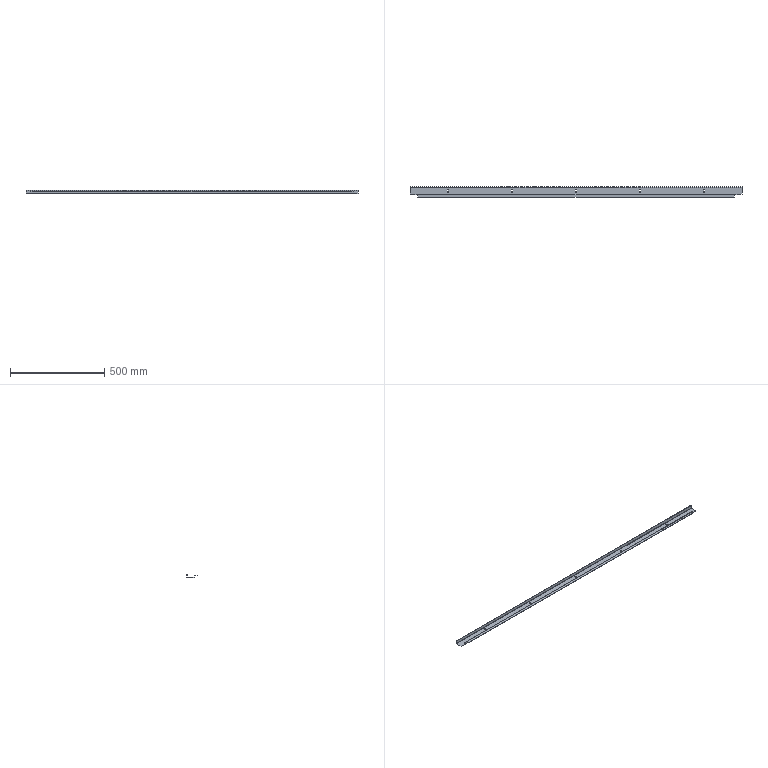Part | SolidWorks | features ICE 5, EdgeFlange 3, FlatPattern 1, SMBaseFlange 1, SheetMetal 1 | 1 solid | 50 faces | box 1760 x 53.5 x 18 mm | volume 208432 mm3 | plane 34 | cylinder 16 | commonest cylinder face diameters 7 x10 2 x3 5 x3
STEP:
#1=CARTESIAN_POINT('',(-855.,-20.,1.));
#2=VERTEX_POINT('',#1);
#3=CARTESIAN_POINT('',(-855.,-20.,10.));
#4=VERTEX_POINT('',#3);
#5=CARTESIAN_POINT('',(-855.,-20.,-1.5));
#6=DIRECTION('',(0.,0.,1.));
#7=VECTOR('',#6,1000.);
#8=LINE('',#5,#7);
#9=EDGE_CURVE('',#2,#4,#8,.T.);
#10=ORIENTED_EDGE('',*,*,#9,.F.);
#11=CARTESIAN_POINT('',(855.,-20.,1.));
#12=VERTEX_POINT('',#11);
#13=CARTESIAN_POINT('',(-880.,-20.,1.));
#14=DIRECTION('',(-1.,0.,0.));
#15=VECTOR('',#14,1000.);
#16=LINE('',#13,#15);
#17=EDGE_CURVE('',#12,#2,#16,.T.);
#18=ORIENTED_EDGE('',*,*,#17,.F.);
#19=CARTESIAN_POINT('',(855.,-20.,10.));
#20=VERTEX_POINT('',#19);
#21=CARTESIAN_POINT('',(855.,-20.,-1.5));
#22=DIRECTION('',(0.,0.,-1.));
#23=VECTOR('',#22,1000.);
#24=LINE('',#21,#23);
#25=EDGE_CURVE('',#20,#12,#24,.T.);
#26=ORIENTED_EDGE('',*,*,#25,.F.);
#27=CARTESIAN_POINT('',(840.,-20.,10.));
#28=VERTEX_POINT('',#27);
#29=CARTESIAN_POINT('',(880.,-20.,10.));
#30=DIRECTION('',(-1.,0.,0.));
#31=VECTOR('',#30,1000.);
#32=LINE('',#29,#31);
#33=EDGE_CURVE('',#20,#28,#32,.T.);
#34=ORIENTED_EDGE('',*,*,#33,.T.);
#35=CARTESIAN_POINT('',(-840.,-20.,10.));
#36=VERTEX_POINT('',#35);
#37=CARTESIAN_POINT('',(-880.,-20.,10.));
#38=DIRECTION('',(1.,0.,0.));
#39=VECTOR('',#38,1000.);
#40=LINE('',#37,#39);
#41=EDGE_CURVE('',#36,#28,#40,.T.);
#42=ORIENTED_EDGE('',*,*,#41,.F.);
#43=CARTESIAN_POINT('',(-880.,-20.,10.));
#44=DIRECTION('',(1.,0.,0.));
#45=VECTOR('',#44,1000.);
#46=LINE('',#43,#45);
#47=EDGE_CURVE('',#4,#36,#46,.T.);
#48=ORIENTED_EDGE('',*,*,#47,.F.);
#49=EDGE_LOOP('',(#10,#18,#26,#34,#42,#48));
#50=FACE_OUTER_BOUND('',#49,.T.);
#51=CARTESIAN_POINT('',(880.,-20.,0.));
#52=DIRECTION('',(0.,1.,0.));
#53=DIRECTION('',(0.,0.,1.));
#54=AXIS2_PLACEMENT_3D('',#51,#52,#53);
#55=PLANE('',#54);
#56=ADVANCED_FACE('',(#50),#55,.F.);
#57=CARTESIAN_POINT('',(-855.,-18.5,1.));
#58=VERTEX_POINT('',#57);
#59=CARTESIAN_POINT('',(855.,-18.5,1.));
#60=VERTEX_POINT('',#59);
#61=CARTESIAN_POINT('',(-880.,-18.5,1.));
#62=DIRECTION('',(1.,0.,0.));
#63=VECTOR('',#62,1000.);
#64=LINE('',#61,#63);
#65=EDGE_CURVE('',#58,#60,#64,.T.);
#66=ORIENTED_EDGE('',*,*,#65,.F.);
#67=CARTESIAN_POINT('',(-855.,-18.5,10.));
#68=VERTEX_POINT('',#67);
#69=CARTESIAN_POINT('',(-855.,-18.5,0.));
#70=DIRECTION('',(0.,0.,1.));
#71=VECTOR('',#70,1000.);
#72=LINE('',#69,#71);
#73=EDGE_CURVE('',#58,#68,#72,.T.);
#74=ORIENTED_EDGE('',*,*,#73,.T.);
#75=CARTESIAN_POINT('',(-840.,-18.5,10.));
#76=VERTEX_POINT('',#75);
#77=CARTESIAN_POINT('',(-880.,-18.5,10.));
#78=DIRECTION('',(1.,0.,0.));
#79=VECTOR('',#78,1000.);
#80=LINE('',#77,#79);
#81=EDGE_CURVE('',#68,#76,#80,.T.);
#82=ORIENTED_EDGE('',*,*,#81,.T.);
#83=CARTESIAN_POINT('',(840.,-18.5,10.));
#84=VERTEX_POINT('',#83);
#85=CARTESIAN_POINT('',(-880.,-18.5,10.));
#86=DIRECTION('',(1.,0.,0.));
#87=VECTOR('',#86,1000.);
#88=LINE('',#85,#87);
#89=EDGE_CURVE('',#76,#84,#88,.T.);
#90=ORIENTED_EDGE('',*,*,#89,.T.);
#91=CARTESIAN_POINT('',(855.,-18.5,10.));
#92=VERTEX_POINT('',#91);
#93=CARTESIAN_POINT('',(840.,-18.5,10.));
#94=DIRECTION('',(1.,0.,0.));
#95=VECTOR('',#94,1000.);
#96=LINE('',#93,#95);
#97=EDGE_CURVE('',#84,#92,#96,.T.);
#98=ORIENTED_EDGE('',*,*,#97,.T.);
#99=CARTESIAN_POINT('',(855.,-18.5,0.));
#100=DIRECTION('',(0.,0.,1.));
#101=VECTOR('',#100,1000.);
#102=LINE('',#99,#101);
#103=EDGE_CURVE('',#60,#92,#102,.T.);
#104=ORIENTED_EDGE('',*,*,#103,.F.);
#105=EDGE_LOOP('',(#66,#74,#82,#90,#98,#104));
#106=FACE_OUTER_BOUND('',#105,.T.);
#107=CARTESIAN_POINT('',(880.,-18.5,0.));
#108=DIRECTION('',(0.,1.,0.));
#109=DIRECTION('',(0.,0.,1.));
#110=AXIS2_PLACEMENT_3D('',#107,#108,#109);
#111=PLANE('',#110);
#112=ADVANCED_FACE('',(#106),#111,.T.);
#113=ORIENTED_EDGE('',*,*,#17,.T.);
#114=CARTESIAN_POINT('',(-855.,-17.5,-1.5));
#115=VERTEX_POINT('',#114);
#116=CARTESIAN_POINT('',(-855.,-17.5,1.));
#117=DIRECTION('',(1.,0.,0.));
#118=DIRECTION('',(0.,0.,1.));
#119=AXIS2_PLACEMENT_3D('',#116,#117,#118);
#120=CIRCLE('',#119,2.5);
#121=EDGE_CURVE('',#2,#115,#120,.T.);
#122=ORIENTED_EDGE('',*,*,#121,.T.);
#123=CARTESIAN_POINT('',(855.,-17.5,-1.5));
#124=VERTEX_POINT('',#123);
#125=CARTESIAN_POINT('',(880.,-17.5,-1.5));
#126=DIRECTION('',(-1.,0.,0.));
#127=VECTOR('',#126,1000.);
#128=LINE('',#125,#127);
#129=EDGE_CURVE('',#124,#115,#128,.T.);
#130=ORIENTED_EDGE('',*,*,#129,.F.);
#131=CARTESIAN_POINT('',(855.,-17.5,1.));
#132=DIRECTION('',(1.,0.,0.));
#133=DIRECTION('',(0.,0.,1.));
#134=AXIS2_PLACEMENT_3D('',#131,#132,#133);
#135=CIRCLE('',#134,2.5);
#136=EDGE_CURVE('',#12,#124,#135,.T.);
#137=ORIENTED_EDGE('',*,*,#136,.F.);
#138=EDGE_LOOP('',(#113,#122,#130,#137));
#139=FACE_OUTER_BOUND('',#138,.T.);
#140=CARTESIAN_POINT('',(880.,-17.5,1.));
#141=DIRECTION('',(1.,0.,0.));
#142=DIRECTION('',(0.,-1.,0.));
#143=AXIS2_PLACEMENT_3D('',#140,#141,#142);
#144=CYLINDRICAL_SURFACE('',#143,2.5);
#145=ADVANCED_FACE('',(#139),#144,.T.);
#146=CARTESIAN_POINT('',(-855.,-17.5,0.));
#147=VERTEX_POINT('',#146);
#148=CARTESIAN_POINT('',(-855.,-17.5,1.));
#149=DIRECTION('',(1.,0.,0.));
#150=DIRECTION('',(0.,0.,1.));
#151=AXIS2_PLACEMENT_3D('',#148,#149,#150);
#152=CIRCLE('',#151,1.);
#153=EDGE_CURVE('',#58,#147,#152,.T.);
#154=ORIENTED_EDGE('',*,*,#153,.F.);
#155=ORIENTED_EDGE('',*,*,#65,.T.);
#156=CARTESIAN_POINT('',(855.,-17.5,0.));
#157=VERTEX_POINT('',#156);
#158=CARTESIAN_POINT('',(855.,-17.5,1.));
#159=DIRECTION('',(1.,0.,0.));
#160=DIRECTION('',(0.,0.,1.));
#161=AXIS2_PLACEMENT_3D('',#158,#159,#160);
#162=CIRCLE('',#161,1.);
#163=EDGE_CURVE('',#60,#157,#162,.T.);
#164=ORIENTED_EDGE('',*,*,#163,.T.);
#165=CARTESIAN_POINT('',(880.,-17.5,0.));
#166=DIRECTION('',(-1.,0.,0.));
#167=VECTOR('',#166,1000.);
#168=LINE('',#165,#167);
#169=EDGE_CURVE('',#157,#147,#168,.T.);
#170=ORIENTED_EDGE('',*,*,#169,.T.);
#171=EDGE_LOOP('',(#154,#155,#164,#170));
#172=FACE_OUTER_BOUND('',#171,.T.);
#173=CARTESIAN_POINT('',(880.,-17.5,1.));
#174=DIRECTION('',(1.,0.,0.));
#175=DIRECTION('',(0.,-1.,0.));
#176=AXIS2_PLACEMENT_3D('',#173,#174,#175);
#177=CYLINDRICAL_SURFACE('',#176,1.);
#178=ADVANCED_FACE('',(#172),#177,.F.);
#179=CARTESIAN_POINT('',(-855.,-17.5,10.));
#180=DIRECTION('',(0.,1.,0.));
#181=VECTOR('',#180,1000.);
#182=LINE('',#179,#181);
#183=EDGE_CURVE('',#4,#68,#182,.T.);
#184=ORIENTED_EDGE('',*,*,#183,.F.);
#185=ORIENTED_EDGE('',*,*,#47,.T.);
#186=CARTESIAN_POINT('',(-840.,-18.5,10.));
#187=DIRECTION('',(0.,-1.,0.));
#188=VECTOR('',#187,1000.);
#189=LINE('',#186,#188);
#190=EDGE_CURVE('',#76,#36,#189,.T.);
#191=ORIENTED_EDGE('',*,*,#190,.F.);
#192=ORIENTED_EDGE('',*,*,#81,.F.);
#193=EDGE_LOOP('',(#184,#185,#191,#192));
#194=FACE_OUTER_BOUND('',#193,.T.);
#195=CARTESIAN_POINT('',(-840.,-18.5,10.));
#196=DIRECTION('',(0.,0.,-1.));
#197=DIRECTION('',(0.,1.,0.));
#198=AXIS2_PLACEMENT_3D('',#195,#196,#197);
#199=PLANE('',#198);
#200=ADVANCED_FACE('',(#194),#199,.F.);
#201=CARTESIAN_POINT('',(840.,-21.,12.5));
#202=VERTEX_POINT('',#201);
#203=CARTESIAN_POINT('',(840.,-21.,10.));
#204=DIRECTION('',(1.,0.,0.));
#205=DIRECTION('',(0.,0.,1.));
#206=AXIS2_PLACEMENT_3D('',#203,#204,#205);
#207=CIRCLE('',#206,2.5);
#208=EDGE_CURVE('',#84,#202,#207,.T.);
#209=ORIENTED_EDGE('',*,*,#208,.F.);
#210=ORIENTED_EDGE('',*,*,#89,.F.);
#211=CARTESIAN_POINT('',(-840.,-21.,12.5));
#212=VERTEX_POINT('',#211);
#213=CARTESIAN_POINT('',(-840.,-21.,10.));
#214=DIRECTION('',(1.,0.,0.));
#215=DIRECTION('',(0.,0.,1.));
#216=AXIS2_PLACEMENT_3D('',#213,#214,#215);
#217=CIRCLE('',#216,2.5);
#218=EDGE_CURVE('',#76,#212,#217,.T.);
#219=ORIENTED_EDGE('',*,*,#218,.T.);
#220=CARTESIAN_POINT('',(880.,-21.,12.5));
#221=DIRECTION('',(1.,0.,0.));
#222=VECTOR('',#221,1000.);
#223=LINE('',#220,#222);
#224=EDGE_CURVE('',#212,#202,#223,.T.);
#225=ORIENTED_EDGE('',*,*,#224,.T.);
#226=EDGE_LOOP('',(#209,#210,#219,#225));
#227=FACE_OUTER_BOUND('',#226,.T.);
#228=CARTESIAN_POINT('',(-880.,-21.,10.));
#229=DIRECTION('',(-1.,0.,0.));
#230=DIRECTION('',(0.,0.,1.));
#231=AXIS2_PLACEMENT_3D('',#228,#229,#230);
#232=CYLINDRICAL_SURFACE('',#231,2.5);
#233=ADVANCED_FACE('',(#227),#232,.T.);
#234=ORIENTED_EDGE('',*,*,#41,.T.);
#235=CARTESIAN_POINT('',(840.,-21.,11.));
#236=VERTEX_POINT('',#235);
#237=CARTESIAN_POINT('',(840.,-21.,10.));
#238=DIRECTION('',(1.,0.,0.));
#239=DIRECTION('',(0.,0.,1.));
#240=AXIS2_PLACEMENT_3D('',#237,#238,#239);
#241=CIRCLE('',#240,1.);
#242=EDGE_CURVE('',#28,#236,#241,.T.);
#243=ORIENTED_EDGE('',*,*,#242,.T.);
#244=CARTESIAN_POINT('',(-840.,-21.,11.));
#245=VERTEX_POINT('',#244);
#246=CARTESIAN_POINT('',(880.,-21.,11.));
#247=DIRECTION('',(-1.,0.,0.));
#248=VECTOR('',#247,1000.);
#249=LINE('',#246,#248);
#250=EDGE_CURVE('',#236,#245,#249,.T.);
#251=ORIENTED_EDGE('',*,*,#250,.T.);
#252=CARTESIAN_POINT('',(-840.,-21.,10.));
#253=DIRECTION('',(1.,0.,0.));
#254=DIRECTION('',(0.,0.,1.));
#255=AXIS2_PLACEMENT_3D('',#252,#253,#254);
#256=CIRCLE('',#255,1.);
#257=EDGE_CURVE('',#36,#245,#256,.T.);
#258=ORIENTED_EDGE('',*,*,#257,.F.);
#259=EDGE_LOOP('',(#234,#243,#251,#258));
#260=FACE_OUTER_BOUND('',#259,.T.);
#261=CARTESIAN_POINT('',(-880.,-21.,10.));
#262=DIRECTION('',(-1.,0.,0.));
#263=DIRECTION('',(0.,0.,1.));
#264=AXIS2_PLACEMENT_3D('',#261,#262,#263);
#265=CYLINDRICAL_SURFACE('',#264,1.);
#266=ADVANCED_FACE('',(#260),#265,.F.);
#267=CARTESIAN_POINT('',(-840.,-33.5,12.5));
#268=VERTEX_POINT('',#267);
#269=CARTESIAN_POINT('',(840.,-33.5,12.5));
#270=VERTEX_POINT('',#269);
#271=CARTESIAN_POINT('',(-880.,-33.5,12.5));
#272=DIRECTION('',(1.,0.,0.));
#273=VECTOR('',#272,1000.);
#274=LINE('',#271,#273);
#275=EDGE_CURVE('',#268,#270,#274,.T.);
#276=ORIENTED_EDGE('',*,*,#275,.T.);
#277=CARTESIAN_POINT('',(840.,-18.5,12.5));
#278=DIRECTION('',(0.,-1.,0.));
#279=VECTOR('',#278,1000.);
#280=LINE('',#277,#279);
#281=EDGE_CURVE('',#202,#270,#280,.T.);
#282=ORIENTED_EDGE('',*,*,#281,.F.);
#283=ORIENTED_EDGE('',*,*,#224,.F.);
#284=CARTESIAN_POINT('',(-840.,-18.5,12.5));
#285=DIRECTION('',(0.,1.,0.));
#286=VECTOR('',#285,1000.);
#287=LINE('',#284,#286);
#288=EDGE_CURVE('',#268,#212,#287,.T.);
#289=ORIENTED_EDGE('',*,*,#288,.F.);
#290=EDGE_LOOP('',(#276,#282,#283,#289));
#291=FACE_OUTER_BOUND('',#290,.T.);
#292=CARTESIAN_POINT('',(-880.,-20.,12.5));
#293=DIRECTION('',(0.,0.,-1.));
#294=DIRECTION('',(0.,1.,0.));
#295=AXIS2_PLACEMENT_3D('',#292,#293,#294);
#296=PLANE('',#295);
#297=ADVANCED_FACE('',(#291),#296,.F.);
#298=CARTESIAN_POINT('',(840.,-33.5,11.));
#299=VERTEX_POINT('',#298);
#300=CARTESIAN_POINT('',(840.,-20.,11.));
#301=DIRECTION('',(0.,1.,0.));
#302=VECTOR('',#301,1000.);
#303=LINE('',#300,#302);
#304=EDGE_CURVE('',#299,#236,#303,.T.);
#305=ORIENTED_EDGE('',*,*,#304,.F.);
#306=CARTESIAN_POINT('',(-840.,-33.5,11.));
#307=VERTEX_POINT('',#306);
#308=CARTESIAN_POINT('',(880.,-33.5,11.));
#309=DIRECTION('',(1.,0.,0.));
#310=VECTOR('',#309,1000.);
#311=LINE('',#308,#310);
#312=EDGE_CURVE('',#307,#299,#311,.T.);
#313=ORIENTED_EDGE('',*,*,#312,.F.);
#314=CARTESIAN_POINT('',(-840.,-20.,11.));
#315=DIRECTION('',(0.,1.,0.));
#316=VECTOR('',#315,1000.);
#317=LINE('',#314,#316);
#318=EDGE_CURVE('',#307,#245,#317,.T.);
#319=ORIENTED_EDGE('',*,*,#318,.T.);
#320=ORIENTED_EDGE('',*,*,#250,.F.);
#321=EDGE_LOOP('',(#305,#313,#319,#320));
#322=FACE_OUTER_BOUND('',#321,.T.);
#323=CARTESIAN_POINT('',(-880.,-20.,11.));
#324=DIRECTION('',(0.,0.,-1.));
#325=DIRECTION('',(0.,1.,0.));
#326=AXIS2_PLACEMENT_3D('',#323,#324,#325);
#327=PLANE('',#326);
#328=ADVANCED_FACE('',(#322),#327,.T.);
#329=ORIENTED_EDGE('',*,*,#312,.T.);
#330=CARTESIAN_POINT('',(840.,-33.5,10.));
#331=DIRECTION('',(0.,0.,-1.));
#332=VECTOR('',#331,1000.);
#333=LINE('',#330,#332);
#334=EDGE_CURVE('',#270,#299,#333,.T.);
#335=ORIENTED_EDGE('',*,*,#334,.F.);
#336=ORIENTED_EDGE('',*,*,#275,.F.);
#337=CARTESIAN_POINT('',(-840.,-33.5,12.5));
#338=DIRECTION('',(0.,0.,1.));
#339=VECTOR('',#338,1000.);
#340=LINE('',#337,#339);
#341=EDGE_CURVE('',#307,#268,#340,.T.);
#342=ORIENTED_EDGE('',*,*,#341,.F.);
#343=EDGE_LOOP('',(#329,#335,#336,#342));
#344=FACE_OUTER_BOUND('',#343,.T.);
#345=CARTESIAN_POINT('',(880.,-33.5,12.5));
#346=DIRECTION('',(0.,1.,0.));
#347=DIRECTION('',(0.,0.,1.));
#348=AXIS2_PLACEMENT_3D('',#345,#346,#347);
#349=PLANE('',#348);
#350=ADVANCED_FACE('',(#344),#349,.F.);
#351=CARTESIAN_POINT('',(676.5,-4.,-1.5));
#352=VERTEX_POINT('',#351);
#353=CARTESIAN_POINT('',(676.5,4.,-1.5));
#354=VERTEX_POINT('',#353);
#355=CARTESIAN_POINT('',(676.5,-4.,-1.5));
#356=DIRECTION('',(0.,1.,0.));
#357=VECTOR('',#356,1000.);
#358=LINE('',#355,#357);
#359=EDGE_CURVE('',#352,#354,#358,.T.);
#360=ORIENTED_EDGE('',*,*,#359,.F.);
#361=CARTESIAN_POINT('',(683.5,-4.,-1.5));
#362=VERTEX_POINT('',#361);
#363=CARTESIAN_POINT('',(680.,-4.,-1.5));
#364=DIRECTION('',(0.,0.,-1.));
#365=DIRECTION('',(-1.,0.,0.));
#366=AXIS2_PLACEMENT_3D('',#363,#364,#365);
#367=CIRCLE('',#366,3.5);
#368=EDGE_CURVE('',#362,#352,#367,.T.);
#369=ORIENTED_EDGE('',*,*,#368,.F.);
#370=CARTESIAN_POINT('',(683.5,4.,-1.5));
#371=VERTEX_POINT('',#370);
#372=CARTESIAN_POINT('',(683.5,-4.,-1.5));
#373=DIRECTION('',(0.,-1.,0.));
#374=VECTOR('',#373,1000.);
#375=LINE('',#372,#374);
#376=EDGE_CURVE('',#371,#362,#375,.T.);
#377=ORIENTED_EDGE('',*,*,#376,.F.);
#378=CARTESIAN_POINT('',(680.,4.,-1.5));
#379=DIRECTION('',(0.,0.,-1.));
#380=DIRECTION('',(-1.,0.,0.));
#381=AXIS2_PLACEMENT_3D('',#378,#379,#380);
#382=CIRCLE('',#381,3.5);
#383=EDGE_CURVE('',#354,#371,#382,.T.);
#384=ORIENTED_EDGE('',*,*,#383,.F.);
#385=EDGE_LOOP('',(#360,#369,#377,#384));
#386=FACE_BOUND('',#385,.T.);
#387=CARTESIAN_POINT('',(336.5,-4.,-1.5));
#388=VERTEX_POINT('',#387);
#389=CARTESIAN_POINT('',(336.5,4.,-1.5));
#390=VERTEX_POINT('',#389);
#391=CARTESIAN_POINT('',(336.5,-4.,-1.5));
#392=DIRECTION('',(0.,1.,0.));
#393=VECTOR('',#392,1000.);
#394=LINE('',#391,#393);
#395=EDGE_CURVE('',#388,#390,#394,.T.);
#396=ORIENTED_EDGE('',*,*,#395,.F.);
#397=CARTESIAN_POINT('',(343.5,-4.,-1.5));
#398=VERTEX_POINT('',#397);
#399=CARTESIAN_POINT('',(340.,-4.,-1.5));
#400=DIRECTION('',(0.,0.,-1.));
#401=DIRECTION('',(-1.,0.,0.));
#402=AXIS2_PLACEMENT_3D('',#399,#400,#401);
#403=CIRCLE('',#402,3.5);
#404=EDGE_CURVE('',#398,#388,#403,.T.);
#405=ORIENTED_EDGE('',*,*,#404,.F.);
#406=CARTESIAN_POINT('',(343.5,4.,-1.5));
#407=VERTEX_POINT('',#406);
#408=CARTESIAN_POINT('',(343.5,-4.,-1.5));
#409=DIRECTION('',(0.,-1.,0.));
#410=VECTOR('',#409,1000.);
#411=LINE('',#408,#410);
#412=EDGE_CURVE('',#407,#398,#411,.T.);
#413=ORIENTED_EDGE('',*,*,#412,.F.);
#414=CARTESIAN_POINT('',(340.,4.,-1.5));
#415=DIRECTION('',(0.,0.,-1.));
#416=DIRECTION('',(-1.,0.,0.));
#417=AXIS2_PLACEMENT_3D('',#414,#415,#416);
#418=CIRCLE('',#417,3.5);
#419=EDGE_CURVE('',#390,#407,#418,.T.);
#420=ORIENTED_EDGE('',*,*,#419,.F.);
#421=EDGE_LOOP('',(#396,#405,#413,#420));
#422=FACE_BOUND('',#421,.T.);
#423=CARTESIAN_POINT('',(-683.5,-4.,-1.5));
#424=VERTEX_POINT('',#423);
#425=CARTESIAN_POINT('',(-683.5,4.,-1.5));
#426=VERTEX_POINT('',#425);
#427=CARTESIAN_POINT('',(-683.5,-4.,-1.5));
#428=DIRECTION('',(0.,1.,0.));
#429=VECTOR('',#428,1000.);
#430=LINE('',#427,#429);
#431=EDGE_CURVE('',#424,#426,#430,.T.);
#432=ORIENTED_EDGE('',*,*,#431,.F.);
#433=CARTESIAN_POINT('',(-676.5,-4.,-1.5));
#434=VERTEX_POINT('',#433);
#435=CARTESIAN_POINT('',(-680.,-4.,-1.5));
#436=DIRECTION('',(0.,0.,-1.));
#437=DIRECTION('',(-1.,0.,0.));
#438=AXIS2_PLACEMENT_3D('',#435,#436,#437);
#439=CIRCLE('',#438,3.5);
#440=EDGE_CURVE('',#434,#424,#439,.T.);
#441=ORIENTED_EDGE('',*,*,#440,.F.);
#442=CARTESIAN_POINT('',(-676.5,4.,-1.5));
#443=VERTEX_POINT('',#442);
#444=CARTESIAN_POINT('',(-676.5,-4.,-1.5));
#445=DIRECTION('',(0.,-1.,0.));
#446=VECTOR('',#445,1000.);
#447=LINE('',#444,#446);
#448=EDGE_CURVE('',#443,#434,#447,.T.);
#449=ORIENTED_EDGE('',*,*,#448,.F.);
#450=CARTESIAN_POINT('',(-680.,4.,-1.5));
#451=DIRECTION('',(0.,0.,-1.));
#452=DIRECTION('',(-1.,0.,0.));
#453=AXIS2_PLACEMENT_3D('',#450,#451,#452);
#454=CIRCLE('',#453,3.5);
#455=EDGE_CURVE('',#426,#443,#454,.T.);
#456=ORIENTED_EDGE('',*,*,#455,.F.);
#457=EDGE_LOOP('',(#432,#441,#449,#456));
#458=FACE_BOUND('',#457,.T.);
#459=CARTESIAN_POINT('',(-343.5,-4.,-1.5));
#460=VERTEX_POINT('',#459);
#461=CARTESIAN_POINT('',(-343.5,4.,-1.5));
#462=VERTEX_POINT('',#461);
#463=CARTESIAN_POINT('',(-343.5,-4.,-1.5));
#464=DIRECTION('',(0.,1.,0.));
#465=VECTOR('',#464,1000.);
#466=LINE('',#463,#465);
#467=EDGE_CURVE('',#460,#462,#466,.T.);
#468=ORIENTED_EDGE('',*,*,#467,.F.);
#469=CARTESIAN_POINT('',(-336.5,-4.,-1.5));
#470=VERTEX_POINT('',#469);
#471=CARTESIAN_POINT('',(-340.,-4.,-1.5));
#472=DIRECTION('',(0.,0.,-1.));
#473=DIRECTION('',(-1.,0.,0.));
#474=AXIS2_PLACEMENT_3D('',#471,#472,#473);
#475=CIRCLE('',#474,3.5);
#476=EDGE_CURVE('',#470,#460,#475,.T.);
#477=ORIENTED_EDGE('',*,*,#476,.F.);
#478=CARTESIAN_POINT('',(-336.5,4.,-1.5));
#479=VERTEX_POINT('',#478);
#480=CARTESIAN_POINT('',(-336.5,-4.,-1.5));
#481=DIRECTION('',(0.,-1.,0.));
#482=VECTOR('',#481,1000.);
#483=LINE('',#480,#482);
#484=EDGE_CURVE('',#479,#470,#483,.T.);
#485=ORIENTED_EDGE('',*,*,#484,.F.);
#486=CARTESIAN_POINT('',(-340.,4.,-1.5));
#487=DIRECTION('',(0.,0.,-1.));
#488=DIRECTION('',(-1.,0.,0.));
#489=AXIS2_PLACEMENT_3D('',#486,#487,#488);
#490=CIRCLE('',#489,3.5);
#491=EDGE_CURVE('',#462,#479,#490,.T.);
#492=ORIENTED_EDGE('',*,*,#491,.F.);
#493=EDGE_LOOP('',(#468,#477,#485,#492));
#494=FACE_BOUND('',#493,.T.);
#495=CARTESIAN_POINT('',(-3.5,-4.,-1.5));
#496=VERTEX_POINT('',#495);
#497=CARTESIAN_POINT('',(-3.5,4.,-1.5));
#498=VERTEX_POINT('',#497);
#499=CARTESIAN_POINT('',(-3.5,-4.,-1.5));
#500=DIRECTION('',(0.,1.,0.));
#501=VECTOR('',#500,1000.);
#502=LINE('',#499,#501);
#503=EDGE_CURVE('',#496,#498,#502,.T.);
#504=ORIENTED_EDGE('',*,*,#503,.F.);
#505=CARTESIAN_POINT('',(3.5,-4.,-1.5));
#506=VERTEX_POINT('',#505);
#507=CARTESIAN_POINT('',(0.,-4.,-1.5));
#508=DIRECTION('',(0.,0.,-1.));
#509=DIRECTION('',(-1.,0.,0.));
#510=AXIS2_PLACEMENT_3D('',#507,#508,#509);
#511=CIRCLE('',#510,3.5);
#512=EDGE_CURVE('',#506,#496,#511,.T.);
#513=ORIENTED_EDGE('',*,*,#512,.F.);
#514=CARTESIAN_POINT('',(3.5,4.,-1.5));
#515=VERTEX_POINT('',#514);
#516=CARTESIAN_POINT('',(3.5,-4.,-1.5));
#517=DIRECTION('',(0.,-1.,0.));
#518=VECTOR('',#517,1000.);
#519=LINE('',#516,#518);
#520=EDGE_CURVE('',#515,#506,#519,.T.);
#521=ORIENTED_EDGE('',*,*,#520,.F.);
#522=CARTESIAN_POINT('',(0.,4.,-1.5));
#523=DIRECTION('',(0.,0.,-1.));
#524=DIRECTION('',(-1.,0.,0.));
#525=AXIS2_PLACEMENT_3D('',#522,#523,#524);
#526=CIRCLE('',#525,3.5);
#527=EDGE_CURVE('',#498,#515,#526,.T.);
#528=ORIENTED_EDGE('',*,*,#527,.F.);
#529=EDGE_LOOP('',(#504,#513,#521,#528));
#530=FACE_BOUND('',#529,.T.);
#531=CARTESIAN_POINT('',(880.,-17.5,-1.5));
#532=VERTEX_POINT('',#531);
#533=CARTESIAN_POINT('',(880.,-17.5,-1.5));
#534=DIRECTION('',(-1.,0.,0.));
#535=VECTOR('',#534,1000.);
#536=LINE('',#533,#535);
#537=EDGE_CURVE('',#532,#124,#536,.T.);
#538=ORIENTED_EDGE('',*,*,#537,.T.);
#539=ORIENTED_EDGE('',*,*,#129,.T.);
#540=CARTESIAN_POINT('',(-880.,-17.5,-1.5));
#541=VERTEX_POINT('',#540);
#542=CARTESIAN_POINT('',(-855.,-17.5,-1.5));
#543=DIRECTION('',(-1.,0.,0.));
#544=VECTOR('',#543,1000.);
#545=LINE('',#542,#544);
#546=EDGE_CURVE('',#115,#541,#545,.T.);
#547=ORIENTED_EDGE('',*,*,#546,.T.);
#548=CARTESIAN_POINT('',(-880.,17.5,-1.5));
#549=VERTEX_POINT('',#548);
#550=CARTESIAN_POINT('',(-880.,20.,-1.5));
#551=DIRECTION('',(0.,-1.,0.));
#552=VECTOR('',#551,1000.);
#553=LINE('',#550,#552);
#554=EDGE_CURVE('',#549,#541,#553,.T.);
#555=ORIENTED_EDGE('',*,*,#554,.F.);
#556=CARTESIAN_POINT('',(880.,17.5,-1.5));
#557=VERTEX_POINT('',#556);
#558=CARTESIAN_POINT('',(-880.,17.5,-1.5));
#559=DIRECTION('',(1.,0.,0.));
#560=VECTOR('',#559,1000.);
#561=LINE('',#558,#560);
#562=EDGE_CURVE('',#549,#557,#561,.T.);
#563=ORIENTED_EDGE('',*,*,#562,.T.);
#564=CARTESIAN_POINT('',(880.,20.,-1.5));
#565=DIRECTION('',(0.,1.,0.));
#566=VECTOR('',#565,1000.);
#567=LINE('',#564,#566);
#568=EDGE_CURVE('',#532,#557,#567,.T.);
#569=ORIENTED_EDGE('',*,*,#568,.F.);
#570=EDGE_LOOP('',(#538,#539,#547,#555,#563,#569));
#571=FACE_OUTER_BOUND('',#570,.T.);
#572=CARTESIAN_POINT('',(880.,-20.,-1.5));
#573=DIRECTION('',(0.,0.,1.));
#574=DIRECTION('',(1.,0.,0.));
#575=AXIS2_PLACEMENT_3D('',#572,#573,#574);
#576=PLANE('',#575);
#577=ADVANCED_FACE('',(#386,#422,#458,#494,#530,#571),#576,.F.);
#578=CARTESIAN_POINT('',(676.5,-4.,0.));
#579=VERTEX_POINT('',#578);
#580=CARTESIAN_POINT('',(683.5,-4.,0.));
#581=VERTEX_POINT('',#580);
#582=CARTESIAN_POINT('',(680.,-4.,0.));
#583=DIRECTION('',(0.,0.,1.));
#584=DIRECTION('',(1.,0.,0.));
#585=AXIS2_PLACEMENT_3D('',#582,#583,#584);
#586=CIRCLE('',#585,3.5);
#587=EDGE_CURVE('',#579,#581,#586,.T.);
#588=ORIENTED_EDGE('',*,*,#587,.F.);
#589=CARTESIAN_POINT('',(676.5,4.,0.));
#590=VERTEX_POINT('',#589);
#591=CARTESIAN_POINT('',(676.5,-20.,0.));
#592=DIRECTION('',(0.,-1.,0.));
#593=VECTOR('',#592,1000.);
#594=LINE('',#591,#593);
#595=EDGE_CURVE('',#590,#579,#594,.T.);
#596=ORIENTED_EDGE('',*,*,#595,.F.);
#597=CARTESIAN_POINT('',(683.5,4.,0.));
#598=VERTEX_POINT('',#597);
#599=CARTESIAN_POINT('',(680.,4.,0.));
#600=DIRECTION('',(0.,0.,1.));
#601=DIRECTION('',(1.,0.,0.));
#602=AXIS2_PLACEMENT_3D('',#599,#600,#601);
#603=CIRCLE('',#602,3.5);
#604=EDGE_CURVE('',#598,#590,#603,.T.);
#605=ORIENTED_EDGE('',*,*,#604,.F.);
#606=CARTESIAN_POINT('',(683.5,-20.,0.));
#607=DIRECTION('',(0.,1.,0.));
#608=VECTOR('',#607,1000.);
#609=LINE('',#606,#608);
#610=EDGE_CURVE('',#581,#598,#609,.T.);
#611=ORIENTED_EDGE('',*,*,#610,.F.);
#612=EDGE_LOOP('',(#588,#596,#605,#611));
#613=FACE_BOUND('',#612,.T.);
#614=CARTESIAN_POINT('',(336.5,-4.,0.));
#615=VERTEX_POINT('',#614);
#616=CARTESIAN_POINT('',(343.5,-4.,0.));
#617=VERTEX_POINT('',#616);
#618=CARTESIAN_POINT('',(340.,-4.,0.));
#619=DIRECTION('',(0.,0.,1.));
#620=DIRECTION('',(1.,0.,0.));
#621=AXIS2_PLACEMENT_3D('',#618,#619,#620);
#622=CIRCLE('',#621,3.5);
#623=EDGE_CURVE('',#615,#617,#622,.T.);
#624=ORIENTED_EDGE('',*,*,#623,.F.);
#625=CARTESIAN_POINT('',(336.5,4.,0.));
#626=VERTEX_POINT('',#625);
#627=CARTESIAN_POINT('',(336.5,-20.,0.));
#628=DIRECTION('',(0.,-1.,0.));
#629=VECTOR('',#628,1000.);
#630=LINE('',#627,#629);
#631=EDGE_CURVE('',#626,#615,#630,.T.);
#632=ORIENTED_EDGE('',*,*,#631,.F.);
#633=CARTESIAN_POINT('',(343.5,4.,0.));
#634=VERTEX_POINT('',#633);
#635=CARTESIAN_POINT('',(340.,4.,0.));
#636=DIRECTION('',(0.,0.,1.));
#637=DIRECTION('',(1.,0.,0.));
#638=AXIS2_PLACEMENT_3D('',#635,#636,#637);
#639=CIRCLE('',#638,3.5);
#640=EDGE_CURVE('',#634,#626,#639,.T.);
#641=ORIENTED_EDGE('',*,*,#640,.F.);
#642=CARTESIAN_POINT('',(343.5,-20.,0.));
#643=DIRECTION('',(0.,1.,0.));
#644=VECTOR('',#643,1000.);
#645=LINE('',#642,#644);
#646=EDGE_CURVE('',#617,#634,#645,.T.);
#647=ORIENTED_EDGE('',*,*,#646,.F.);
#648=EDGE_LOOP('',(#624,#632,#641,#647));
#649=FACE_BOUND('',#648,.T.);
#650=CARTESIAN_POINT('',(-683.5,-4.,0.));
#651=VERTEX_POINT('',#650);
#652=CARTESIAN_POINT('',(-676.5,-4.,0.));
#653=VERTEX_POINT('',#652);
#654=CARTESIAN_POINT('',(-680.,-4.,0.));
#655=DIRECTION('',(0.,0.,1.));
#656=DIRECTION('',(1.,0.,0.));
#657=AXIS2_PLACEMENT_3D('',#654,#655,#656);
#658=CIRCLE('',#657,3.5);
#659=EDGE_CURVE('',#651,#653,#658,.T.);
#660=ORIENTED_EDGE('',*,*,#659,.F.);
#661=CARTESIAN_POINT('',(-683.5,4.,0.));
#662=VERTEX_POINT('',#661);
#663=CARTESIAN_POINT('',(-683.5,-20.,0.));
#664=DIRECTION('',(0.,-1.,0.));
#665=VECTOR('',#664,1000.);
#666=LINE('',#663,#665);
#667=EDGE_CURVE('',#662,#651,#666,.T.);
#668=ORIENTED_EDGE('',*,*,#667,.F.);
#669=CARTESIAN_POINT('',(-676.5,4.,0.));
#670=VERTEX_POINT('',#669);
#671=CARTESIAN_POINT('',(-680.,4.,0.));
#672=DIRECTION('',(0.,0.,1.));
#673=DIRECTION('',(1.,0.,0.));
#674=AXIS2_PLACEMENT_3D('',#671,#672,#673);
#675=CIRCLE('',#674,3.5);
#676=EDGE_CURVE('',#670,#662,#675,.T.);
#677=ORIENTED_EDGE('',*,*,#676,.F.);
#678=CARTESIAN_POINT('',(-676.5,-20.,0.));
#679=DIRECTION('',(0.,1.,0.));
#680=VECTOR('',#679,1000.);
#681=LINE('',#678,#680);
#682=EDGE_CURVE('',#653,#670,#681,.T.);
#683=ORIENTED_EDGE('',*,*,#682,.F.);
#684=EDGE_LOOP('',(#660,#668,#677,#683));
#685=FACE_BOUND('',#684,.T.);
#686=CARTESIAN_POINT('',(-343.5,-4.,0.));
#687=VERTEX_POINT('',#686);
#688=CARTESIAN_POINT('',(-336.5,-4.,0.));
#689=VERTEX_POINT('',#688);
#690=CARTESIAN_POINT('',(-340.,-4.,0.));
#691=DIRECTION('',(0.,0.,1.));
#692=DIRECTION('',(1.,0.,0.));
#693=AXIS2_PLACEMENT_3D('',#690,#691,#692);
#694=CIRCLE('',#693,3.5);
#695=EDGE_CURVE('',#687,#689,#694,.T.);
#696=ORIENTED_EDGE('',*,*,#695,.F.);
#697=CARTESIAN_POINT('',(-343.5,4.,0.));
#698=VERTEX_POINT('',#697);
#699=CARTESIAN_POINT('',(-343.5,-20.,0.));
#700=DIRECTION('',(0.,-1.,0.));
#701=VECTOR('',#700,1000.);
#702=LINE('',#699,#701);
#703=EDGE_CURVE('',#698,#687,#702,.T.);
#704=ORIENTED_EDGE('',*,*,#703,.F.);
#705=CARTESIAN_POINT('',(-336.5,4.,0.));
#706=VERTEX_POINT('',#705);
#707=CARTESIAN_POINT('',(-340.,4.,0.));
#708=DIRECTION('',(0.,0.,1.));
#709=DIRECTION('',(1.,0.,0.));
#710=AXIS2_PLACEMENT_3D('',#707,#708,#709);
#711=CIRCLE('',#710,3.5);
#712=EDGE_CURVE('',#706,#698,#711,.T.);
#713=ORIENTED_EDGE('',*,*,#712,.F.);
#714=CARTESIAN_POINT('',(-336.5,-20.,0.));
#715=DIRECTION('',(0.,1.,0.));
#716=VECTOR('',#715,1000.);
#717=LINE('',#714,#716);
#718=EDGE_CURVE('',#689,#706,#717,.T.);
#719=ORIENTED_EDGE('',*,*,#718,.F.);
#720=EDGE_LOOP('',(#696,#704,#713,#719));
#721=FACE_BOUND('',#720,.T.);
#722=CARTESIAN_POINT('',(-3.5,-4.,0.));
#723=VERTEX_POINT('',#722);
#724=CARTESIAN_POINT('',(3.5,-4.,0.));
#725=VERTEX_POINT('',#724);
#726=CARTESIAN_POINT('',(0.,-4.,0.));
#727=DIRECTION('',(0.,0.,1.));
#728=DIRECTION('',(1.,0.,0.));
#729=AXIS2_PLACEMENT_3D('',#726,#727,#728);
#730=CIRCLE('',#729,3.5);
#731=EDGE_CURVE('',#723,#725,#730,.T.);
#732=ORIENTED_EDGE('',*,*,#731,.F.);
#733=CARTESIAN_POINT('',(-3.5,4.,0.));
#734=VERTEX_POINT('',#733);
#735=CARTESIAN_POINT('',(-3.5,-20.,0.));
#736=DIRECTION('',(0.,-1.,0.));
#737=VECTOR('',#736,1000.);
#738=LINE('',#735,#737);
#739=EDGE_CURVE('',#734,#723,#738,.T.);
#740=ORIENTED_EDGE('',*,*,#739,.F.);
#741=CARTESIAN_POINT('',(3.5,4.,0.));
#742=VERTEX_POINT('',#741);
#743=CARTESIAN_POINT('',(0.,4.,0.));
#744=DIRECTION('',(0.,0.,1.));
#745=DIRECTION('',(1.,0.,0.));
#746=AXIS2_PLACEMENT_3D('',#743,#744,#745);
#747=CIRCLE('',#746,3.5);
#748=EDGE_CURVE('',#742,#734,#747,.T.);
#749=ORIENTED_EDGE('',*,*,#748,.F.);
#750=CARTESIAN_POINT('',(3.5,-20.,0.));
#751=DIRECTION('',(0.,1.,0.));
#752=VECTOR('',#751,1000.);
#753=LINE('',#750,#752);
#754=EDGE_CURVE('',#725,#742,#753,.T.);
#755=ORIENTED_EDGE('',*,*,#754,.F.);
#756=EDGE_LOOP('',(#732,#740,#749,#755));
#757=FACE_BOUND('',#756,.T.);
#758=CARTESIAN_POINT('',(-880.,17.5,0.));
#759=VERTEX_POINT('',#758);
#760=CARTESIAN_POINT('',(-880.,-17.5,0.));
#761=VERTEX_POINT('',#760);
#762=CARTESIAN_POINT('',(-880.,20.,0.));
#763=DIRECTION('',(0.,-1.,0.));
#764=VECTOR('',#763,1000.);
#765=LINE('',#762,#764);
#766=EDGE_CURVE('',#759,#761,#765,.T.);
#767=ORIENTED_EDGE('',*,*,#766,.T.);
#768=CARTESIAN_POINT('',(880.,-17.5,0.));
#769=DIRECTION('',(-1.,0.,0.));
#770=VECTOR('',#769,1000.);
#771=LINE('',#768,#770);
#772=EDGE_CURVE('',#147,#761,#771,.T.);
#773=ORIENTED_EDGE('',*,*,#772,.F.);
#774=ORIENTED_EDGE('',*,*,#169,.F.);
#775=CARTESIAN_POINT('',(880.,-17.5,0.));
#776=VERTEX_POINT('',#775);
#777=CARTESIAN_POINT('',(880.,-17.5,0.));
#778=DIRECTION('',(-1.,0.,0.));
#779=VECTOR('',#778,1000.);
#780=LINE('',#777,#779);
#781=EDGE_CURVE('',#776,#157,#780,.T.);
#782=ORIENTED_EDGE('',*,*,#781,.F.);
#783=CARTESIAN_POINT('',(880.,17.5,0.));
#784=VERTEX_POINT('',#783);
#785=CARTESIAN_POINT('',(880.,20.,0.));
#786=DIRECTION('',(0.,1.,0.));
#787=VECTOR('',#786,1000.);
#788=LINE('',#785,#787);
#789=EDGE_CURVE('',#776,#784,#788,.T.);
#790=ORIENTED_EDGE('',*,*,#789,.T.);
#791=CARTESIAN_POINT('',(-880.,17.5,0.));
#792=DIRECTION('',(1.,0.,0.));
#793=VECTOR('',#792,1000.);
#794=LINE('',#791,#793);
#795=EDGE_CURVE('',#759,#784,#794,.T.);
#796=ORIENTED_EDGE('',*,*,#795,.F.);
#797=EDGE_LOOP('',(#767,#773,#774,#782,#790,#796));
#798=FACE_OUTER_BOUND('',#797,.T.);
#799=CARTESIAN_POINT('',(880.,-20.,0.));
#800=DIRECTION('',(0.,0.,1.));
#801=DIRECTION('',(1.,0.,0.));
#802=AXIS2_PLACEMENT_3D('',#799,#800,#801);
#803=PLANE('',#802);
#804=ADVANCED_FACE('',(#613,#649,#685,#721,#757,#798),#803,.T.);
#805=ORIENTED_EDGE('',*,*,#789,.F.);
#806=CARTESIAN_POINT('',(880.,-17.5,0.));
#807=DIRECTION('',(0.,0.,-1.));
#808=VECTOR('',#807,1000.);
#809=LINE('',#806,#808);
#810=EDGE_CURVE('',#776,#532,#809,.T.);
#811=ORIENTED_EDGE('',*,*,#810,.T.);
#812=ORIENTED_EDGE('',*,*,#568,.T.);
#813=CARTESIAN_POINT('',(880.,17.5,0.));
#814=DIRECTION('',(0.,0.,-1.));
#815=VECTOR('',#814,1000.);
#816=LINE('',#813,#815);
#817=EDGE_CURVE('',#784,#557,#816,.T.);
#818=ORIENTED_EDGE('',*,*,#817,.F.);
#819=EDGE_LOOP('',(#805,#811,#812,#818));
#820=FACE_OUTER_BOUND('',#819,.T.);
#821=CARTESIAN_POINT('',(880.,20.,-1.5));
#822=DIRECTION('',(1.,0.,0.));
#823=DIRECTION('',(0.,0.,-1.));
#824=AXIS2_PLACEMENT_3D('',#821,#822,#823);
#825=PLANE('',#824);
#826=ADVANCED_FACE('',(#820),#825,.T.);
#827=CARTESIAN_POINT('',(-880.,-17.5,0.));
#828=DIRECTION('',(0.,0.,-1.));
#829=VECTOR('',#828,1000.);
#830=LINE('',#827,#829);
#831=EDGE_CURVE('',#761,#541,#830,.T.);
#832=ORIENTED_EDGE('',*,*,#831,.F.);
#833=ORIENTED_EDGE('',*,*,#766,.F.);
#834=CARTESIAN_POINT('',(-880.,17.5,0.));
#835=DIRECTION('',(0.,0.,-1.));
#836=VECTOR('',#835,1000.);
#837=LINE('',#834,#836);
#838=EDGE_CURVE('',#759,#549,#837,.T.);
#839=ORIENTED_EDGE('',*,*,#838,.T.);
#840=ORIENTED_EDGE('',*,*,#554,.T.);
#841=EDGE_LOOP('',(#832,#833,#839,#840));
#842=FACE_OUTER_BOUND('',#841,.T.);
#843=CARTESIAN_POINT('',(-880.,20.,-1.5));
#844=DIRECTION('',(-1.,0.,0.));
#845=DIRECTION('',(0.,0.,1.));
#846=AXIS2_PLACEMENT_3D('',#843,#844,#845);
#847=PLANE('',#846);
#848=ADVANCED_FACE('',(#842),#847,.T.);
#849=CARTESIAN_POINT('',(880.,18.5,1.));
#850=VERTEX_POINT('',#849);
#851=CARTESIAN_POINT('',(880.,20.,1.));
#852=VERTEX_POINT('',#851);
#853=CARTESIAN_POINT('',(880.,20.,1.));
#854=DIRECTION('',(0.,1.,0.));
#855=VECTOR('',#854,1000.);
#856=LINE('',#853,#855);
#857=EDGE_CURVE('',#850,#852,#856,.T.);
#858=ORIENTED_EDGE('',*,*,#857,.F.);
#859=CARTESIAN_POINT('',(880.,17.5,1.));
#860=DIRECTION('',(1.,0.,0.));
#861=DIRECTION('',(0.,0.,1.));
#862=AXIS2_PLACEMENT_3D('',#859,#860,#861);
#863=CIRCLE('',#862,1.);
#864=EDGE_CURVE('',#784,#850,#863,.T.);
#865=ORIENTED_EDGE('',*,*,#864,.F.);
#866=ORIENTED_EDGE('',*,*,#817,.T.);
#867=CARTESIAN_POINT('',(880.,17.5,1.));
#868=DIRECTION('',(1.,0.,0.));
#869=DIRECTION('',(0.,0.,1.));
#870=AXIS2_PLACEMENT_3D('',#867,#868,#869);
#871=CIRCLE('',#870,2.5);
#872=EDGE_CURVE('',#557,#852,#871,.T.);
#873=ORIENTED_EDGE('',*,*,#872,.T.);
#874=EDGE_LOOP('',(#858,#865,#866,#873));
#875=FACE_OUTER_BOUND('',#874,.T.);
#876=CARTESIAN_POINT('',(880.,17.5,1.));
#877=DIRECTION('',(1.,0.,0.));
#878=DIRECTION('',(0.,0.,-1.));
#879=AXIS2_PLACEMENT_3D('',#876,#877,#878);
#880=PLANE('',#879);
#881=ADVANCED_FACE('',(#875),#880,.T.);
#882=CARTESIAN_POINT('',(-880.,18.5,1.));
#883=VERTEX_POINT('',#882);
#884=CARTESIAN_POINT('',(-880.,17.5,1.));
#885=DIRECTION('',(-1.,0.,0.));
#886=DIRECTION('',(0.,0.,1.));
#887=AXIS2_PLACEMENT_3D('',#884,#885,#886);
#888=CIRCLE('',#887,1.);
#889=EDGE_CURVE('',#883,#759,#888,.T.);
#890=ORIENTED_EDGE('',*,*,#889,.F.);
#891=CARTESIAN_POINT('',(-880.,20.,1.));
#892=VERTEX_POINT('',#891);
#893=CARTESIAN_POINT('',(-880.,18.5,1.));
#894=DIRECTION('',(0.,1.,0.));
#895=VECTOR('',#894,1000.);
#896=LINE('',#893,#895);
#897=EDGE_CURVE('',#883,#892,#896,.T.);
#898=ORIENTED_EDGE('',*,*,#897,.T.);
#899=CARTESIAN_POINT('',(-880.,17.5,1.));
#900=DIRECTION('',(-1.,0.,0.));
#901=DIRECTION('',(0.,0.,1.));
#902=AXIS2_PLACEMENT_3D('',#899,#900,#901);
#903=CIRCLE('',#902,2.5);
#904=EDGE_CURVE('',#892,#549,#903,.T.);
#905=ORIENTED_EDGE('',*,*,#904,.T.);
#906=ORIENTED_EDGE('',*,*,#838,.F.);
#907=EDGE_LOOP('',(#890,#898,#905,#906));
#908=FACE_OUTER_BOUND('',#907,.T.);
#909=CARTESIAN_POINT('',(-880.,17.5,1.));
#910=DIRECTION('',(1.,0.,0.));
#911=DIRECTION('',(0.,0.,-1.));
#912=AXIS2_PLACEMENT_3D('',#909,#910,#911);
#913=PLANE('',#912);
#914=ADVANCED_FACE('',(#908),#913,.F.);
#915=ORIENTED_EDGE('',*,*,#562,.F.);
#916=ORIENTED_EDGE('',*,*,#904,.F.);
#917=CARTESIAN_POINT('',(880.,20.,1.));
#918=DIRECTION('',(1.,0.,0.));
#919=VECTOR('',#918,1000.);
#920=LINE('',#917,#919);
#921=EDGE_CURVE('',#892,#852,#920,.T.);
#922=ORIENTED_EDGE('',*,*,#921,.T.);
#923=ORIENTED_EDGE('',*,*,#872,.F.);
#924=EDGE_LOOP('',(#915,#916,#922,#923));
#925=FACE_OUTER_BOUND('',#924,.T.);
#926=CARTESIAN_POINT('',(-880.,17.5,1.));
#927=DIRECTION('',(-1.,0.,0.));
#928=DIRECTION('',(0.,1.,0.));
#929=AXIS2_PLACEMENT_3D('',#926,#927,#928);
#930=CYLINDRICAL_SURFACE('',#929,2.5);
#931=ADVANCED_FACE('',(#925),#930,.T.);
#932=ORIENTED_EDGE('',*,*,#795,.T.);
#933=ORIENTED_EDGE('',*,*,#864,.T.);
#934=CARTESIAN_POINT('',(880.,18.5,1.));
#935=DIRECTION('',(-1.,0.,0.));
#936=VECTOR('',#935,1000.);
#937=LINE('',#934,#936);
#938=EDGE_CURVE('',#850,#883,#937,.T.);
#939=ORIENTED_EDGE('',*,*,#938,.T.);
#940=ORIENTED_EDGE('',*,*,#889,.T.);
#941=EDGE_LOOP('',(#932,#933,#939,#940));
#942=FACE_OUTER_BOUND('',#941,.T.);
#943=CARTESIAN_POINT('',(-880.,17.5,1.));
#944=DIRECTION('',(-1.,0.,0.));
#945=DIRECTION('',(0.,1.,0.));
#946=AXIS2_PLACEMENT_3D('',#943,#944,#945);
#947=CYLINDRICAL_SURFACE('',#946,1.);
#948=ADVANCED_FACE('',(#942),#947,.F.);
#949=ORIENTED_EDGE('',*,*,#857,.T.);
#950=CARTESIAN_POINT('',(880.,20.,16.5));
#951=VERTEX_POINT('',#950);
#952=CARTESIAN_POINT('',(880.,20.,16.5));
#953=DIRECTION('',(0.,0.,-1.));
#954=VECTOR('',#953,1000.);
#955=LINE('',#952,#954);
#956=EDGE_CURVE('',#951,#852,#955,.T.);
#957=ORIENTED_EDGE('',*,*,#956,.F.);
#958=CARTESIAN_POINT('',(880.,18.5,16.5));
#959=VERTEX_POINT('',#958);
#960=CARTESIAN_POINT('',(880.,20.,16.5));
#961=DIRECTION('',(0.,-1.,0.));
#962=VECTOR('',#961,1000.);
#963=LINE('',#960,#962);
#964=EDGE_CURVE('',#951,#959,#963,.T.);
#965=ORIENTED_EDGE('',*,*,#964,.T.);
#966=CARTESIAN_POINT('',(880.,18.5,0.));
#967=DIRECTION('',(0.,0.,-1.));
#968=VECTOR('',#967,1000.);
#969=LINE('',#966,#968);
#970=EDGE_CURVE('',#959,#850,#969,.T.);
#971=ORIENTED_EDGE('',*,*,#970,.T.);
#972=EDGE_LOOP('',(#949,#957,#965,#971));
#973=FACE_OUTER_BOUND('',#972,.T.);
#974=CARTESIAN_POINT('',(880.,20.,0.));
#975=DIRECTION('',(-1.,0.,0.));
#976=DIRECTION('',(0.,0.,1.));
#977=AXIS2_PLACEMENT_3D('',#974,#975,#976);
#978=PLANE('',#977);
#979=ADVANCED_FACE('',(#973),#978,.F.);
#980=ORIENTED_EDGE('',*,*,#897,.F.);
#981=CARTESIAN_POINT('',(-880.,18.5,16.5));
#982=VERTEX_POINT('',#981);
#983=CARTESIAN_POINT('',(-880.,18.5,16.5));
#984=DIRECTION('',(0.,0.,1.));
#985=VECTOR('',#984,1000.);
#986=LINE('',#983,#985);
#987=EDGE_CURVE('',#883,#982,#986,.T.);
#988=ORIENTED_EDGE('',*,*,#987,.T.);
#989=CARTESIAN_POINT('',(-880.,20.,16.5));
#990=VERTEX_POINT('',#989);
#991=CARTESIAN_POINT('',(-880.,20.,16.5));
#992=DIRECTION('',(0.,-1.,0.));
#993=VECTOR('',#992,1000.);
#994=LINE('',#991,#993);
#995=EDGE_CURVE('',#990,#982,#994,.T.);
#996=ORIENTED_EDGE('',*,*,#995,.F.);
#997=CARTESIAN_POINT('',(-880.,20.,16.5));
#998=DIRECTION('',(0.,0.,1.));
#999=VECTOR('',#998,1000.);
#1000=LINE('',#997,#999);
#1001=EDGE_CURVE('',#892,#990,#1000,.T.);
#1002=ORIENTED_EDGE('',*,*,#1001,.F.);
#1003=EDGE_LOOP('',(#980,#988,#996,#1002));
#1004=FACE_OUTER_BOUND('',#1003,.T.);
#1005=CARTESIAN_POINT('',(-880.,20.,16.5));
#1006=DIRECTION('',(1.,0.,0.));
#1007=DIRECTION('',(0.,0.,-1.));
#1008=AXIS2_PLACEMENT_3D('',#1005,#1006,#1007);
#1009=PLANE('',#1008);
#1010=ADVANCED_FACE('',(#1004),#1009,.F.);
#1011=ORIENTED_EDGE('',*,*,#921,.F.);
#1012=ORIENTED_EDGE('',*,*,#1001,.T.);
#1013=CARTESIAN_POINT('',(880.,20.,16.5));
#1014=DIRECTION('',(1.,0.,0.));
#1015=VECTOR('',#1014,1000.);
#1016=LINE('',#1013,#1015);
#1017=EDGE_CURVE('',#990,#951,#1016,.T.);
#1018=ORIENTED_EDGE('',*,*,#1017,.T.);
#1019=ORIENTED_EDGE('',*,*,#956,.T.);
#1020=EDGE_LOOP('',(#1011,#1012,#1018,#1019));
#1021=FACE_OUTER_BOUND('',#1020,.T.);
#1022=CARTESIAN_POINT('',(880.,20.,16.5));
#1023=DIRECTION('',(0.,-1.,0.));
#1024=DIRECTION('',(0.,0.,-1.));
#1025=AXIS2_PLACEMENT_3D('',#1022,#1023,#1024);
#1026=PLANE('',#1025);
#1027=ADVANCED_FACE('',(#1021),#1026,.F.);
#1028=ORIENTED_EDGE('',*,*,#987,.F.);
#1029=ORIENTED_EDGE('',*,*,#938,.F.);
#1030=ORIENTED_EDGE('',*,*,#970,.F.);
#1031=CARTESIAN_POINT('',(880.,18.5,16.5));
#1032=DIRECTION('',(1.,0.,0.));
#1033=VECTOR('',#1032,1000.);
#1034=LINE('',#1031,#1033);
#1035=EDGE_CURVE('',#982,#959,#1034,.T.);
#1036=ORIENTED_EDGE('',*,*,#1035,.F.);
#1037=EDGE_LOOP('',(#1028,#1029,#1030,#1036));
#1038=FACE_OUTER_BOUND('',#1037,.T.);
#1039=CARTESIAN_POINT('',(880.,18.5,16.5));
#1040=DIRECTION('',(0.,-1.,0.));
#1041=DIRECTION('',(0.,0.,-1.));
#1042=AXIS2_PLACEMENT_3D('',#1039,#1040,#1041);
#1043=PLANE('',#1042);
#1044=ADVANCED_FACE('',(#1038),#1043,.T.);
#1045=ORIENTED_EDGE('',*,*,#1035,.T.);
#1046=ORIENTED_EDGE('',*,*,#964,.F.);
#1047=ORIENTED_EDGE('',*,*,#1017,.F.);
#1048=ORIENTED_EDGE('',*,*,#995,.T.);
#1049=EDGE_LOOP('',(#1045,#1046,#1047,#1048));
#1050=FACE_OUTER_BOUND('',#1049,.T.);
#1051=CARTESIAN_POINT('',(880.,20.,16.5));
#1052=DIRECTION('',(0.,0.,-1.));
#1053=DIRECTION('',(0.,1.,0.));
#1054=AXIS2_PLACEMENT_3D('',#1051,#1052,#1053);
#1055=PLANE('',#1054);
#1056=ADVANCED_FACE('',(#1050),#1055,.F.);
#1057=ORIENTED_EDGE('',*,*,#731,.T.);
#1058=CARTESIAN_POINT('',(3.5,-4.,0.5));
#1059=DIRECTION('',(0.,0.,-1.));
#1060=VECTOR('',#1059,1000.);
#1061=LINE('',#1058,#1060);
#1062=EDGE_CURVE('',#725,#506,#1061,.T.);
#1063=ORIENTED_EDGE('',*,*,#1062,.T.);
#1064=ORIENTED_EDGE('',*,*,#512,.T.);
#1065=CARTESIAN_POINT('',(-3.5,-4.,0.5));
#1066=DIRECTION('',(0.,0.,-1.));
#1067=VECTOR('',#1066,1000.);
#1068=LINE('',#1065,#1067);
#1069=EDGE_CURVE('',#723,#496,#1068,.T.);
#1070=ORIENTED_EDGE('',*,*,#1069,.F.);
#1071=EDGE_LOOP('',(#1057,#1063,#1064,#1070));
#1072=FACE_OUTER_BOUND('',#1071,.T.);
#1073=CARTESIAN_POINT('',(0.,-4.,0.5));
#1074=DIRECTION('',(0.,0.,-1.));
#1075=DIRECTION('',(-1.,0.,0.));
#1076=AXIS2_PLACEMENT_3D('',#1073,#1074,#1075);
#1077=CYLINDRICAL_SURFACE('',#1076,3.5);
#1078=ADVANCED_FACE('',(#1072),#1077,.F.);
#1079=ORIENTED_EDGE('',*,*,#754,.T.);
#1080=CARTESIAN_POINT('',(3.5,4.,0.5));
#1081=DIRECTION('',(0.,0.,-1.));
#1082=VECTOR('',#1081,1000.);
#1083=LINE('',#1080,#1082);
#1084=EDGE_CURVE('',#742,#515,#1083,.T.);
#1085=ORIENTED_EDGE('',*,*,#1084,.T.);
#1086=ORIENTED_EDGE('',*,*,#520,.T.);
#1087=ORIENTED_EDGE('',*,*,#1062,.F.);
#1088=EDGE_LOOP('',(#1079,#1085,#1086,#1087));
#1089=FACE_OUTER_BOUND('',#1088,.T.);
#1090=CARTESIAN_POINT('',(3.5,-4.,0.5));
#1091=DIRECTION('',(1.,0.,0.));
#1092=DIRECTION('',(0.,1.,0.));
#1093=AXIS2_PLACEMENT_3D('',#1090,#1091,#1092);
#1094=PLANE('',#1093);
#1095=ADVANCED_FACE('',(#1089),#1094,.F.);
#1096=ORIENTED_EDGE('',*,*,#748,.T.);
#1097=CARTESIAN_POINT('',(-3.5,4.,0.5));
#1098=DIRECTION('',(0.,0.,-1.));
#1099=VECTOR('',#1098,1000.);
#1100=LINE('',#1097,#1099);
#1101=EDGE_CURVE('',#734,#498,#1100,.T.);
#1102=ORIENTED_EDGE('',*,*,#1101,.T.);
#1103=ORIENTED_EDGE('',*,*,#527,.T.);
#1104=ORIENTED_EDGE('',*,*,#1084,.F.);
#1105=EDGE_LOOP('',(#1096,#1102,#1103,#1104));
#1106=FACE_OUTER_BOUND('',#1105,.T.);
#1107=CARTESIAN_POINT('',(0.,4.,0.5));
#1108=DIRECTION('',(0.,0.,-1.));
#1109=DIRECTION('',(-1.,0.,0.));
#1110=AXIS2_PLACEMENT_3D('',#1107,#1108,#1109);
#1111=CYLINDRICAL_SURFACE('',#1110,3.5);
#1112=ADVANCED_FACE('',(#1106),#1111,.F.);
#1113=ORIENTED_EDGE('',*,*,#739,.T.);
#1114=ORIENTED_EDGE('',*,*,#1069,.T.);
#1115=ORIENTED_EDGE('',*,*,#503,.T.);
#1116=ORIENTED_EDGE('',*,*,#1101,.F.);
#1117=EDGE_LOOP('',(#1113,#1114,#1115,#1116));
#1118=FACE_OUTER_BOUND('',#1117,.T.);
#1119=CARTESIAN_POINT('',(-3.5,-4.,0.5));
#1120=DIRECTION('',(-1.,0.,0.));
#1121=DIRECTION('',(0.,-1.,0.));
#1122=AXIS2_PLACEMENT_3D('',#1119,#1120,#1121);
#1123=PLANE('',#1122);
#1124=ADVANCED_FACE('',(#1118),#1123,.F.);
#1125=ORIENTED_EDGE('',*,*,#695,.T.);
#1126=CARTESIAN_POINT('',(-336.5,-4.,0.5));
#1127=DIRECTION('',(0.,0.,-1.));
#1128=VECTOR('',#1127,1000.);
#1129=LINE('',#1126,#1128);
#1130=EDGE_CURVE('',#689,#470,#1129,.T.);
#1131=ORIENTED_EDGE('',*,*,#1130,.T.);
#1132=ORIENTED_EDGE('',*,*,#476,.T.);
#1133=CARTESIAN_POINT('',(-343.5,-4.,0.5));
#1134=DIRECTION('',(0.,0.,-1.));
#1135=VECTOR('',#1134,1000.);
#1136=LINE('',#1133,#1135);
#1137=EDGE_CURVE('',#687,#460,#1136,.T.);
#1138=ORIENTED_EDGE('',*,*,#1137,.F.);
#1139=EDGE_LOOP('',(#1125,#1131,#1132,#1138));
#1140=FACE_OUTER_BOUND('',#1139,.T.);
#1141=CARTESIAN_POINT('',(-340.,-4.,0.5));
#1142=DIRECTION('',(0.,0.,-1.));
#1143=DIRECTION('',(-1.,0.,0.));
#1144=AXIS2_PLACEMENT_3D('',#1141,#1142,#1143);
#1145=CYLINDRICAL_SURFACE('',#1144,3.5);
#1146=ADVANCED_FACE('',(#1140),#1145,.F.);
#1147=ORIENTED_EDGE('',*,*,#718,.T.);
#1148=CARTESIAN_POINT('',(-336.5,4.,0.5));
#1149=DIRECTION('',(0.,0.,-1.));
#1150=VECTOR('',#1149,1000.);
#1151=LINE('',#1148,#1150);
#1152=EDGE_CURVE('',#706,#479,#1151,.T.);
#1153=ORIENTED_EDGE('',*,*,#1152,.T.);
#1154=ORIENTED_EDGE('',*,*,#484,.T.);
#1155=ORIENTED_EDGE('',*,*,#1130,.F.);
#1156=EDGE_LOOP('',(#1147,#1153,#1154,#1155));
#1157=FACE_OUTER_BOUND('',#1156,.T.);
#1158=CARTESIAN_POINT('',(-336.5,-4.,0.5));
#1159=DIRECTION('',(1.,0.,0.));
#1160=DIRECTION('',(0.,0.,-1.));
#1161=AXIS2_PLACEMENT_3D('',#1158,#1159,#1160);
#1162=PLANE('',#1161);
#1163=ADVANCED_FACE('',(#1157),#1162,.F.);
#1164=ORIENTED_EDGE('',*,*,#712,.T.);
#1165=CARTESIAN_POINT('',(-343.5,4.,0.5));
#1166=DIRECTION('',(0.,0.,-1.));
#1167=VECTOR('',#1166,1000.);
#1168=LINE('',#1165,#1167);
#1169=EDGE_CURVE('',#698,#462,#1168,.T.);
#1170=ORIENTED_EDGE('',*,*,#1169,.T.);
#1171=ORIENTED_EDGE('',*,*,#491,.T.);
#1172=ORIENTED_EDGE('',*,*,#1152,.F.);
#1173=EDGE_LOOP('',(#1164,#1170,#1171,#1172));
#1174=FACE_OUTER_BOUND('',#1173,.T.);
#1175=CARTESIAN_POINT('',(-340.,4.,0.5));
#1176=DIRECTION('',(0.,0.,-1.));
#1177=DIRECTION('',(-1.,0.,0.));
#1178=AXIS2_PLACEMENT_3D('',#1175,#1176,#1177);
#1179=CYLINDRICAL_SURFACE('',#1178,3.5);
#1180=ADVANCED_FACE('',(#1174),#1179,.F.);
#1181=ORIENTED_EDGE('',*,*,#703,.T.);
#1182=ORIENTED_EDGE('',*,*,#1137,.T.);
#1183=ORIENTED_EDGE('',*,*,#467,.T.);
#1184=ORIENTED_EDGE('',*,*,#1169,.F.);
#1185=EDGE_LOOP('',(#1181,#1182,#1183,#1184));
#1186=FACE_OUTER_BOUND('',#1185,.T.);
#1187=CARTESIAN_POINT('',(-343.5,-4.,0.5));
#1188=DIRECTION('',(-1.,0.,0.));
#1189=DIRECTION('',(0.,0.,1.));
#1190=AXIS2_PLACEMENT_3D('',#1187,#1188,#1189);
#1191=PLANE('',#1190);
#1192=ADVANCED_FACE('',(#1186),#1191,.F.);
#1193=ORIENTED_EDGE('',*,*,#659,.T.);
#1194=CARTESIAN_POINT('',(-676.5,-4.,0.5));
#1195=DIRECTION('',(0.,0.,-1.));
#1196=VECTOR('',#1195,1000.);
#1197=LINE('',#1194,#1196);
#1198=EDGE_CURVE('',#653,#434,#1197,.T.);
#1199=ORIENTED_EDGE('',*,*,#1198,.T.);
#1200=ORIENTED_EDGE('',*,*,#440,.T.);
#1201=CARTESIAN_POINT('',(-683.5,-4.,0.5));
#1202=DIRECTION('',(0.,0.,-1.));
#1203=VECTOR('',#1202,1000.);
#1204=LINE('',#1201,#1203);
#1205=EDGE_CURVE('',#651,#424,#1204,.T.);
#1206=ORIENTED_EDGE('',*,*,#1205,.F.);
#1207=EDGE_LOOP('',(#1193,#1199,#1200,#1206));
#1208=FACE_OUTER_BOUND('',#1207,.T.);
#1209=CARTESIAN_POINT('',(-680.,-4.,0.5));
#1210=DIRECTION('',(0.,0.,-1.));
#1211=DIRECTION('',(-1.,0.,0.));
#1212=AXIS2_PLACEMENT_3D('',#1209,#1210,#1211);
#1213=CYLINDRICAL_SURFACE('',#1212,3.5);
#1214=ADVANCED_FACE('',(#1208),#1213,.F.);
#1215=ORIENTED_EDGE('',*,*,#682,.T.);
#1216=CARTESIAN_POINT('',(-676.5,4.,0.5));
#1217=DIRECTION('',(0.,0.,-1.));
#1218=VECTOR('',#1217,1000.);
#1219=LINE('',#1216,#1218);
#1220=EDGE_CURVE('',#670,#443,#1219,.T.);
#1221=ORIENTED_EDGE('',*,*,#1220,.T.);
#1222=ORIENTED_EDGE('',*,*,#448,.T.);
#1223=ORIENTED_EDGE('',*,*,#1198,.F.);
#1224=EDGE_LOOP('',(#1215,#1221,#1222,#1223));
#1225=FACE_OUTER_BOUND('',#1224,.T.);
#1226=CARTESIAN_POINT('',(-676.5,-4.,0.5));
#1227=DIRECTION('',(1.,0.,0.));
#1228=DIRECTION('',(0.,0.,-1.));
#1229=AXIS2_PLACEMENT_3D('',#1226,#1227,#1228);
#1230=PLANE('',#1229);
#1231=ADVANCED_FACE('',(#1225),#1230,.F.);
#1232=ORIENTED_EDGE('',*,*,#676,.T.);
#1233=CARTESIAN_POINT('',(-683.5,4.,0.5));
#1234=DIRECTION('',(0.,0.,-1.));
#1235=VECTOR('',#1234,1000.);
#1236=LINE('',#1233,#1235);
#1237=EDGE_CURVE('',#662,#426,#1236,.T.);
#1238=ORIENTED_EDGE('',*,*,#1237,.T.);
#1239=ORIENTED_EDGE('',*,*,#455,.T.);
#1240=ORIENTED_EDGE('',*,*,#1220,.F.);
#1241=EDGE_LOOP('',(#1232,#1238,#1239,#1240));
#1242=FACE_OUTER_BOUND('',#1241,.T.);
#1243=CARTESIAN_POINT('',(-680.,4.,0.5));
#1244=DIRECTION('',(0.,0.,-1.));
#1245=DIRECTION('',(-1.,0.,0.));
#1246=AXIS2_PLACEMENT_3D('',#1243,#1244,#1245);
#1247=CYLINDRICAL_SURFACE('',#1246,3.5);
#1248=ADVANCED_FACE('',(#1242),#1247,.F.);
#1249=ORIENTED_EDGE('',*,*,#667,.T.);
#1250=ORIENTED_EDGE('',*,*,#1205,.T.);
#1251=ORIENTED_EDGE('',*,*,#431,.T.);
#1252=ORIENTED_EDGE('',*,*,#1237,.F.);
#1253=EDGE_LOOP('',(#1249,#1250,#1251,#1252));
#1254=FACE_OUTER_BOUND('',#1253,.T.);
#1255=CARTESIAN_POINT('',(-683.5,-4.,0.5));
#1256=DIRECTION('',(-1.,0.,0.));
#1257=DIRECTION('',(0.,0.,1.));
#1258=AXIS2_PLACEMENT_3D('',#1255,#1256,#1257);
#1259=PLANE('',#1258);
#1260=ADVANCED_FACE('',(#1254),#1259,.F.);
#1261=ORIENTED_EDGE('',*,*,#623,.T.);
#1262=CARTESIAN_POINT('',(343.5,-4.,0.5));
#1263=DIRECTION('',(0.,0.,-1.));
#1264=VECTOR('',#1263,1000.);
#1265=LINE('',#1262,#1264);
#1266=EDGE_CURVE('',#617,#398,#1265,.T.);
#1267=ORIENTED_EDGE('',*,*,#1266,.T.);
#1268=ORIENTED_EDGE('',*,*,#404,.T.);
#1269=CARTESIAN_POINT('',(336.5,-4.,0.5));
#1270=DIRECTION('',(0.,0.,-1.));
#1271=VECTOR('',#1270,1000.);
#1272=LINE('',#1269,#1271);
#1273=EDGE_CURVE('',#615,#388,#1272,.T.);
#1274=ORIENTED_EDGE('',*,*,#1273,.F.);
#1275=EDGE_LOOP('',(#1261,#1267,#1268,#1274));
#1276=FACE_OUTER_BOUND('',#1275,.T.);
#1277=CARTESIAN_POINT('',(340.,-4.,0.5));
#1278=DIRECTION('',(0.,0.,-1.));
#1279=DIRECTION('',(-1.,0.,0.));
#1280=AXIS2_PLACEMENT_3D('',#1277,#1278,#1279);
#1281=CYLINDRICAL_SURFACE('',#1280,3.5);
#1282=ADVANCED_FACE('',(#1276),#1281,.F.);
#1283=ORIENTED_EDGE('',*,*,#646,.T.);
#1284=CARTESIAN_POINT('',(343.5,4.,0.5));
#1285=DIRECTION('',(0.,0.,-1.));
#1286=VECTOR('',#1285,1000.);
#1287=LINE('',#1284,#1286);
#1288=EDGE_CURVE('',#634,#407,#1287,.T.);
#1289=ORIENTED_EDGE('',*,*,#1288,.T.);
#1290=ORIENTED_EDGE('',*,*,#412,.T.);
#1291=ORIENTED_EDGE('',*,*,#1266,.F.);
#1292=EDGE_LOOP('',(#1283,#1289,#1290,#1291));
#1293=FACE_OUTER_BOUND('',#1292,.T.);
#1294=CARTESIAN_POINT('',(343.5,-4.,0.5));
#1295=DIRECTION('',(1.,0.,0.));
#1296=DIRECTION('',(0.,0.,-1.));
#1297=AXIS2_PLACEMENT_3D('',#1294,#1295,#1296);
#1298=PLANE('',#1297);
#1299=ADVANCED_FACE('',(#1293),#1298,.F.);
#1300=ORIENTED_EDGE('',*,*,#640,.T.);
#1301=CARTESIAN_POINT('',(336.5,4.,0.5));
#1302=DIRECTION('',(0.,0.,-1.));
#1303=VECTOR('',#1302,1000.);
#1304=LINE('',#1301,#1303);
#1305=EDGE_CURVE('',#626,#390,#1304,.T.);
#1306=ORIENTED_EDGE('',*,*,#1305,.T.);
#1307=ORIENTED_EDGE('',*,*,#419,.T.);
#1308=ORIENTED_EDGE('',*,*,#1288,.F.);
#1309=EDGE_LOOP('',(#1300,#1306,#1307,#1308));
#1310=FACE_OUTER_BOUND('',#1309,.T.);
#1311=CARTESIAN_POINT('',(340.,4.,0.5));
#1312=DIRECTION('',(0.,0.,-1.));
#1313=DIRECTION('',(-1.,0.,0.));
#1314=AXIS2_PLACEMENT_3D('',#1311,#1312,#1313);
#1315=CYLINDRICAL_SURFACE('',#1314,3.5);
#1316=ADVANCED_FACE('',(#1310),#1315,.F.);
#1317=ORIENTED_EDGE('',*,*,#631,.T.);
#1318=ORIENTED_EDGE('',*,*,#1273,.T.);
#1319=ORIENTED_EDGE('',*,*,#395,.T.);
#1320=ORIENTED_EDGE('',*,*,#1305,.F.);
#1321=EDGE_LOOP('',(#1317,#1318,#1319,#1320));
#1322=FACE_OUTER_BOUND('',#1321,.T.);
#1323=CARTESIAN_POINT('',(336.5,-4.,0.5));
#1324=DIRECTION('',(-1.,0.,0.));
#1325=DIRECTION('',(0.,0.,1.));
#1326=AXIS2_PLACEMENT_3D('',#1323,#1324,#1325);
#1327=PLANE('',#1326);
#1328=ADVANCED_FACE('',(#1322),#1327,.F.);
#1329=ORIENTED_EDGE('',*,*,#587,.T.);
#1330=CARTESIAN_POINT('',(683.5,-4.,0.5));
#1331=DIRECTION('',(0.,0.,-1.));
#1332=VECTOR('',#1331,1000.);
#1333=LINE('',#1330,#1332);
#1334=EDGE_CURVE('',#581,#362,#1333,.T.);
#1335=ORIENTED_EDGE('',*,*,#1334,.T.);
#1336=ORIENTED_EDGE('',*,*,#368,.T.);
#1337=CARTESIAN_POINT('',(676.5,-4.,0.5));
#1338=DIRECTION('',(0.,0.,-1.));
#1339=VECTOR('',#1338,1000.);
#1340=LINE('',#1337,#1339);
#1341=EDGE_CURVE('',#579,#352,#1340,.T.);
#1342=ORIENTED_EDGE('',*,*,#1341,.F.);
#1343=EDGE_LOOP('',(#1329,#1335,#1336,#1342));
#1344=FACE_OUTER_BOUND('',#1343,.T.);
#1345=CARTESIAN_POINT('',(680.,-4.,0.5));
#1346=DIRECTION('',(0.,0.,-1.));
#1347=DIRECTION('',(-1.,0.,0.));
#1348=AXIS2_PLACEMENT_3D('',#1345,#1346,#1347);
#1349=CYLINDRICAL_SURFACE('',#1348,3.5);
#1350=ADVANCED_FACE('',(#1344),#1349,.F.);
#1351=ORIENTED_EDGE('',*,*,#610,.T.);
#1352=CARTESIAN_POINT('',(683.5,4.,0.5));
#1353=DIRECTION('',(0.,0.,-1.));
#1354=VECTOR('',#1353,1000.);
#1355=LINE('',#1352,#1354);
#1356=EDGE_CURVE('',#598,#371,#1355,.T.);
#1357=ORIENTED_EDGE('',*,*,#1356,.T.);
#1358=ORIENTED_EDGE('',*,*,#376,.T.);
#1359=ORIENTED_EDGE('',*,*,#1334,.F.);
#1360=EDGE_LOOP('',(#1351,#1357,#1358,#1359));
#1361=FACE_OUTER_BOUND('',#1360,.T.);
#1362=CARTESIAN_POINT('',(683.5,-4.,0.5));
#1363=DIRECTION('',(1.,0.,0.));
#1364=DIRECTION('',(0.,0.,-1.));
#1365=AXIS2_PLACEMENT_3D('',#1362,#1363,#1364);
#1366=PLANE('',#1365);
#1367=ADVANCED_FACE('',(#1361),#1366,.F.);
#1368=ORIENTED_EDGE('',*,*,#604,.T.);
#1369=CARTESIAN_POINT('',(676.5,4.,0.5));
#1370=DIRECTION('',(0.,0.,-1.));
#1371=VECTOR('',#1370,1000.);
#1372=LINE('',#1369,#1371);
#1373=EDGE_CURVE('',#590,#354,#1372,.T.);
#1374=ORIENTED_EDGE('',*,*,#1373,.T.);
#1375=ORIENTED_EDGE('',*,*,#383,.T.);
#1376=ORIENTED_EDGE('',*,*,#1356,.F.);
#1377=EDGE_LOOP('',(#1368,#1374,#1375,#1376));
#1378=FACE_OUTER_BOUND('',#1377,.T.);
#1379=CARTESIAN_POINT('',(680.,4.,0.5));
#1380=DIRECTION('',(0.,0.,-1.));
#1381=DIRECTION('',(-1.,0.,0.));
#1382=AXIS2_PLACEMENT_3D('',#1379,#1380,#1381);
#1383=CYLINDRICAL_SURFACE('',#1382,3.5);
#1384=ADVANCED_FACE('',(#1378),#1383,.F.);
#1385=ORIENTED_EDGE('',*,*,#595,.T.);
#1386=ORIENTED_EDGE('',*,*,#1341,.T.);
#1387=ORIENTED_EDGE('',*,*,#359,.T.);
#1388=ORIENTED_EDGE('',*,*,#1373,.F.);
#1389=EDGE_LOOP('',(#1385,#1386,#1387,#1388));
#1390=FACE_OUTER_BOUND('',#1389,.T.);
#1391=CARTESIAN_POINT('',(676.5,-4.,0.5));
#1392=DIRECTION('',(-1.,0.,0.));
#1393=DIRECTION('',(0.,0.,1.));
#1394=AXIS2_PLACEMENT_3D('',#1391,#1392,#1393);
#1395=PLANE('',#1394);
#1396=ADVANCED_FACE('',(#1390),#1395,.F.);
#1397=ORIENTED_EDGE('',*,*,#190,.T.);
#1398=ORIENTED_EDGE('',*,*,#257,.T.);
#1399=ORIENTED_EDGE('',*,*,#318,.F.);
#1400=ORIENTED_EDGE('',*,*,#341,.T.);
#1401=ORIENTED_EDGE('',*,*,#288,.T.);
#1402=ORIENTED_EDGE('',*,*,#218,.F.);
#1403=EDGE_LOOP('',(#1397,#1398,#1399,#1400,#1401,#1402));
#1404=FACE_OUTER_BOUND('',#1403,.T.);
#1405=CARTESIAN_POINT('',(-840.,-33.5,10.));
#1406=DIRECTION('',(-1.,0.,0.));
#1407=DIRECTION('',(0.,0.,1.));
#1408=AXIS2_PLACEMENT_3D('',#1405,#1406,#1407);
#1409=PLANE('',#1408);
#1410=ADVANCED_FACE('',(#1404),#1409,.T.);
#1411=ORIENTED_EDGE('',*,*,#208,.T.);
#1412=ORIENTED_EDGE('',*,*,#281,.T.);
#1413=ORIENTED_EDGE('',*,*,#334,.T.);
#1414=ORIENTED_EDGE('',*,*,#304,.T.);
#1415=ORIENTED_EDGE('',*,*,#242,.F.);
#1416=CARTESIAN_POINT('',(840.,-18.5,10.));
#1417=DIRECTION('',(0.,1.,0.));
#1418=VECTOR('',#1417,1000.);
#1419=LINE('',#1416,#1418);
#1420=EDGE_CURVE('',#28,#84,#1419,.T.);
#1421=ORIENTED_EDGE('',*,*,#1420,.T.);
#1422=EDGE_LOOP('',(#1411,#1412,#1413,#1414,#1415,#1421));
#1423=FACE_OUTER_BOUND('',#1422,.T.);
#1424=CARTESIAN_POINT('',(840.,-33.5,10.));
#1425=DIRECTION('',(-1.,0.,0.));
#1426=DIRECTION('',(0.,0.,1.));
#1427=AXIS2_PLACEMENT_3D('',#1424,#1425,#1426);
#1428=PLANE('',#1427);
#1429=ADVANCED_FACE('',(#1423),#1428,.F.);
#1430=ORIENTED_EDGE('',*,*,#33,.F.);
#1431=CARTESIAN_POINT('',(855.,-18.5,10.));
#1432=DIRECTION('',(0.,1.,0.));
#1433=VECTOR('',#1432,1000.);
#1434=LINE('',#1431,#1433);
#1435=EDGE_CURVE('',#20,#92,#1434,.T.);
#1436=ORIENTED_EDGE('',*,*,#1435,.T.);
#1437=ORIENTED_EDGE('',*,*,#97,.F.);
#1438=ORIENTED_EDGE('',*,*,#1420,.F.);
#1439=EDGE_LOOP('',(#1430,#1436,#1437,#1438));
#1440=FACE_OUTER_BOUND('',#1439,.T.);
#1441=CARTESIAN_POINT('',(840.,-18.5,10.));
#1442=DIRECTION('',(0.,0.,-1.));
#1443=DIRECTION('',(0.,1.,0.));
#1444=AXIS2_PLACEMENT_3D('',#1441,#1442,#1443);
#1445=PLANE('',#1444);
#1446=ADVANCED_FACE('',(#1440),#1445,.F.);
#1447=CARTESIAN_POINT('',(855.,-17.5,-1.5));
#1448=DIRECTION('',(0.,0.,1.));
#1449=VECTOR('',#1448,1000.);
#1450=LINE('',#1447,#1449);
#1451=EDGE_CURVE('',#124,#157,#1450,.T.);
#1452=ORIENTED_EDGE('',*,*,#1451,.F.);
#1453=ORIENTED_EDGE('',*,*,#537,.F.);
#1454=ORIENTED_EDGE('',*,*,#810,.F.);
#1455=ORIENTED_EDGE('',*,*,#781,.T.);
#1456=EDGE_LOOP('',(#1452,#1453,#1454,#1455));
#1457=FACE_OUTER_BOUND('',#1456,.T.);
#1458=CARTESIAN_POINT('',(855.,-17.5,-1.5));
#1459=DIRECTION('',(0.,1.,0.));
#1460=DIRECTION('',(0.,0.,1.));
#1461=AXIS2_PLACEMENT_3D('',#1458,#1459,#1460);
#1462=PLANE('',#1461);
#1463=ADVANCED_FACE('',(#1457),#1462,.F.);
#1464=ORIENTED_EDGE('',*,*,#136,.T.);
#1465=ORIENTED_EDGE('',*,*,#1451,.T.);
#1466=ORIENTED_EDGE('',*,*,#163,.F.);
#1467=ORIENTED_EDGE('',*,*,#103,.T.);
#1468=ORIENTED_EDGE('',*,*,#1435,.F.);
#1469=ORIENTED_EDGE('',*,*,#25,.T.);
#1470=EDGE_LOOP('',(#1464,#1465,#1466,#1467,#1468,#1469));
#1471=FACE_OUTER_BOUND('',#1470,.T.);
#1472=CARTESIAN_POINT('',(855.,-20.,-1.5));
#1473=DIRECTION('',(-1.,0.,0.));
#1474=DIRECTION('',(0.,0.,1.));
#1475=AXIS2_PLACEMENT_3D('',#1472,#1473,#1474);
#1476=PLANE('',#1475);
#1477=ADVANCED_FACE('',(#1471),#1476,.F.);
#1478=ORIENTED_EDGE('',*,*,#831,.T.);
#1479=ORIENTED_EDGE('',*,*,#546,.F.);
#1480=CARTESIAN_POINT('',(-855.,-17.5,-1.5));
#1481=DIRECTION('',(0.,0.,-1.));
#1482=VECTOR('',#1481,1000.);
#1483=LINE('',#1480,#1482);
#1484=EDGE_CURVE('',#147,#115,#1483,.T.);
#1485=ORIENTED_EDGE('',*,*,#1484,.F.);
#1486=ORIENTED_EDGE('',*,*,#772,.T.);
#1487=EDGE_LOOP('',(#1478,#1479,#1485,#1486));
#1488=FACE_OUTER_BOUND('',#1487,.T.);
#1489=CARTESIAN_POINT('',(-855.,-17.5,-1.5));
#1490=DIRECTION('',(0.,1.,0.));
#1491=DIRECTION('',(0.,0.,1.));
#1492=AXIS2_PLACEMENT_3D('',#1489,#1490,#1491);
#1493=PLANE('',#1492);
#1494=ADVANCED_FACE('',(#1488),#1493,.F.);
#1495=ORIENTED_EDGE('',*,*,#9,.T.);
#1496=ORIENTED_EDGE('',*,*,#183,.T.);
#1497=ORIENTED_EDGE('',*,*,#73,.F.);
#1498=ORIENTED_EDGE('',*,*,#153,.T.);
#1499=ORIENTED_EDGE('',*,*,#1484,.T.);
#1500=ORIENTED_EDGE('',*,*,#121,.F.);
#1501=EDGE_LOOP('',(#1495,#1496,#1497,#1498,#1499,#1500));
#1502=FACE_OUTER_BOUND('',#1501,.T.);
#1503=CARTESIAN_POINT('',(-855.,-20.,-1.5));
#1504=DIRECTION('',(-1.,0.,0.));
#1505=DIRECTION('',(0.,0.,1.));
#1506=AXIS2_PLACEMENT_3D('',#1503,#1504,#1505);
#1507=PLANE('',#1506);
#1508=ADVANCED_FACE('',(#1502),#1507,.T.);
#1509=CLOSED_SHELL('',(#56,#112,#145,#178,#200,#233,#266,#297,#328,#350,#577,#804,#826,#848,#881,#914,#931,#948,#979,#1010,#1027,#1044,#1056,#1078,#1095,#1112,#1124,#1146,#1163,#1180,#1192,#1214,#1231,#1248,#1260,#1282,#1299,#1316,#1328,#1350,#1367,#1384,#1396,#1410,#1429,#1446,#1463,#1477,#1494,#1508));
#1510=MANIFOLD_SOLID_BREP('',#1509);
#1511=CARTESIAN_POINT('',(0.,0.,0.));
#1512=DIRECTION('',(0.,0.,1.));
#1513=DIRECTION('',(1.,0.,0.));
#1514=AXIS2_PLACEMENT_3D('',#1511,#1512,#1513);
#1515=(LENGTH_UNIT()NAMED_UNIT(*)SI_UNIT(.MILLI.,.METRE.));
#1516=UNCERTAINTY_MEASURE_WITH_UNIT(LENGTH_MEASURE(0.00001),#1515,'','');
#1517=(NAMED_UNIT(*)PLANE_ANGLE_UNIT()SI_UNIT($,.RADIAN.));
#1518=(NAMED_UNIT(*)SI_UNIT($,.STERADIAN.)SOLID_ANGLE_UNIT());
#1519=(GEOMETRIC_REPRESENTATION_CONTEXT(3)GLOBAL_UNCERTAINTY_ASSIGNED_CONTEXT((#1516))GLOBAL_UNIT_ASSIGNED_CONTEXT((#1515,#1517,#1518))REPRESENTATION_CONTEXT('',''));
#1520=ADVANCED_BREP_SHAPE_REPRESENTATION('',(#1510,#1514),#1519);